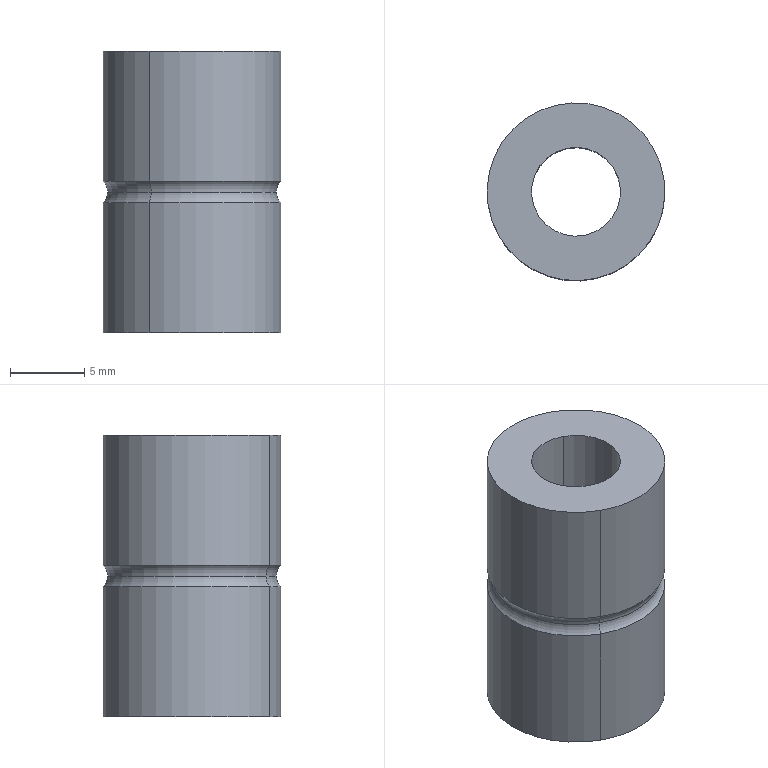Part | SolidWorks | features BaseBody 1 | 1 solid | 12 faces | box 12 x 12 x 19 mm | volume 1601 mm3 | cylinder 6 | torus 4 | plane 2 | commonest cylinder face diameters 12 x4 6 x2
STEP:
#1=CARTESIAN_POINT('',(-798.033,661.045,523.732));
#2=VERTEX_POINT('',#1);
#3=CARTESIAN_POINT('',(-792.229,671.548,523.732));
#4=VERTEX_POINT('',#3);
#5=CARTESIAN_POINT('',(-795.131,666.297,523.732));
#6=DIRECTION('',(0.,0.,1.));
#7=DIRECTION('',(-0.4837,-0.8752,0.));
#8=AXIS2_PLACEMENT_3D('',#5,#6,#7);
#9=CIRCLE('',#8,6.);
#10=EDGE_CURVE('',#2,#4,#9,.T.);
#11=ORIENTED_EDGE('',*,*,#10,.T.);
#12=CARTESIAN_POINT('',(-792.229,671.548,532.518));
#13=VERTEX_POINT('',#12);
#14=CARTESIAN_POINT('',(-792.229,671.548,532.518));
#15=DIRECTION('',(0.,0.,-1.));
#16=VECTOR('',#15,1000.);
#17=LINE('',#14,#16);
#18=EDGE_CURVE('',#13,#4,#17,.T.);
#19=ORIENTED_EDGE('',*,*,#18,.F.);
#20=CARTESIAN_POINT('',(-798.033,661.045,532.518));
#21=VERTEX_POINT('',#20);
#22=CARTESIAN_POINT('',(-795.131,666.297,532.518));
#23=DIRECTION('',(0.,0.,-1.));
#24=DIRECTION('',(0.4837,0.8752,0.));
#25=AXIS2_PLACEMENT_3D('',#22,#23,#24);
#26=CIRCLE('',#25,6.);
#27=EDGE_CURVE('',#13,#21,#26,.T.);
#28=ORIENTED_EDGE('',*,*,#27,.T.);
#29=CARTESIAN_POINT('',(-798.033,661.045,523.732));
#30=DIRECTION('',(0.,0.,1.));
#31=VECTOR('',#30,1000.);
#32=LINE('',#29,#31);
#33=EDGE_CURVE('',#2,#21,#32,.T.);
#34=ORIENTED_EDGE('',*,*,#33,.F.);
#35=EDGE_LOOP('',(#11,#19,#28,#34));
#36=FACE_OUTER_BOUND('',#35,.T.);
#37=CARTESIAN_POINT('',(-795.131,666.297,541.232));
#38=DIRECTION('',(0.,0.,-1.));
#39=DIRECTION('',(-0.4837,-0.8752,0.));
#40=AXIS2_PLACEMENT_3D('',#37,#38,#39);
#41=CYLINDRICAL_SURFACE('',#40,6.);
#42=ADVANCED_FACE('',(#36),#41,.T.);
#43=ORIENTED_EDGE('',*,*,#18,.T.);
#44=CARTESIAN_POINT('',(-795.131,666.297,523.732));
#45=DIRECTION('',(0.,0.,1.));
#46=DIRECTION('',(0.4837,0.8752,0.));
#47=AXIS2_PLACEMENT_3D('',#44,#45,#46);
#48=CIRCLE('',#47,6.);
#49=EDGE_CURVE('',#4,#2,#48,.T.);
#50=ORIENTED_EDGE('',*,*,#49,.T.);
#51=ORIENTED_EDGE('',*,*,#33,.T.);
#52=CARTESIAN_POINT('',(-795.131,666.297,532.518));
#53=DIRECTION('',(0.,0.,-1.));
#54=DIRECTION('',(-0.4837,-0.8752,0.));
#55=AXIS2_PLACEMENT_3D('',#52,#53,#54);
#56=CIRCLE('',#55,6.);
#57=EDGE_CURVE('',#21,#13,#56,.T.);
#58=ORIENTED_EDGE('',*,*,#57,.T.);
#59=EDGE_LOOP('',(#43,#50,#51,#58));
#60=FACE_OUTER_BOUND('',#59,.T.);
#61=CARTESIAN_POINT('',(-795.131,666.297,541.232));
#62=DIRECTION('',(0.,0.,-1.));
#63=DIRECTION('',(-0.4837,-0.8752,0.));
#64=AXIS2_PLACEMENT_3D('',#61,#62,#63);
#65=CYLINDRICAL_SURFACE('',#64,6.);
#66=ADVANCED_FACE('',(#60),#65,.T.);
#67=CARTESIAN_POINT('',(-792.374,671.286,533.232));
#68=VERTEX_POINT('',#67);
#69=CARTESIAN_POINT('',(-791.89,672.161,533.232));
#70=DIRECTION('',(0.8752,-0.4837,0.));
#71=DIRECTION('',(-0.4837,-0.8752,0.));
#72=AXIS2_PLACEMENT_3D('',#69,#70,#71);
#73=CIRCLE('',#72,1.);
#74=EDGE_CURVE('',#68,#13,#73,.T.);
#75=ORIENTED_EDGE('',*,*,#74,.T.);
#76=ORIENTED_EDGE('',*,*,#57,.F.);
#77=CARTESIAN_POINT('',(-797.888,661.308,533.232));
#78=VERTEX_POINT('',#77);
#79=CARTESIAN_POINT('',(-798.371,660.433,533.232));
#80=DIRECTION('',(0.8752,-0.4837,0.));
#81=DIRECTION('',(0.3386,0.6127,-0.7141));
#82=AXIS2_PLACEMENT_3D('',#79,#80,#81);
#83=CIRCLE('',#82,1.);
#84=EDGE_CURVE('',#21,#78,#83,.T.);
#85=ORIENTED_EDGE('',*,*,#84,.T.);
#86=CARTESIAN_POINT('',(-795.131,666.297,533.232));
#87=DIRECTION('',(0.,0.,1.));
#88=DIRECTION('',(0.4837,0.8752,0.));
#89=AXIS2_PLACEMENT_3D('',#86,#87,#88);
#90=CIRCLE('',#89,5.7);
#91=EDGE_CURVE('',#68,#78,#90,.T.);
#92=ORIENTED_EDGE('',*,*,#91,.F.);
#93=EDGE_LOOP('',(#75,#76,#85,#92));
#94=FACE_OUTER_BOUND('',#93,.T.);
#95=CARTESIAN_POINT('',(-795.131,666.297,533.232));
#96=DIRECTION('',(0.,0.,-1.));
#97=DIRECTION('',(-0.4837,-0.8752,0.));
#98=AXIS2_PLACEMENT_3D('',#95,#96,#97);
#99=TOROIDAL_SURFACE('',#98,6.7,1.);
#100=ADVANCED_FACE('',(#94),#99,.F.);
#101=CARTESIAN_POINT('',(-792.229,671.548,533.946));
#102=VERTEX_POINT('',#101);
#103=CARTESIAN_POINT('',(-798.033,661.045,533.946));
#104=VERTEX_POINT('',#103);
#105=CARTESIAN_POINT('',(-795.131,666.297,533.946));
#106=DIRECTION('',(0.,0.,1.));
#107=DIRECTION('',(0.4837,0.8752,0.));
#108=AXIS2_PLACEMENT_3D('',#105,#106,#107);
#109=CIRCLE('',#108,6.);
#110=EDGE_CURVE('',#102,#104,#109,.T.);
#111=ORIENTED_EDGE('',*,*,#110,.F.);
#112=CARTESIAN_POINT('',(-791.89,672.161,533.232));
#113=DIRECTION('',(-0.8752,0.4837,0.));
#114=DIRECTION('',(-0.4837,-0.8752,0.));
#115=AXIS2_PLACEMENT_3D('',#112,#113,#114);
#116=CIRCLE('',#115,1.);
#117=EDGE_CURVE('',#68,#102,#116,.T.);
#118=ORIENTED_EDGE('',*,*,#117,.F.);
#119=ORIENTED_EDGE('',*,*,#91,.T.);
#120=CARTESIAN_POINT('',(-798.371,660.433,533.232));
#121=DIRECTION('',(-0.8752,0.4837,0.));
#122=DIRECTION('',(0.3386,0.6127,0.7141));
#123=AXIS2_PLACEMENT_3D('',#120,#121,#122);
#124=CIRCLE('',#123,1.);
#125=EDGE_CURVE('',#104,#78,#124,.T.);
#126=ORIENTED_EDGE('',*,*,#125,.F.);
#127=EDGE_LOOP('',(#111,#118,#119,#126));
#128=FACE_OUTER_BOUND('',#127,.T.);
#129=CARTESIAN_POINT('',(-795.131,666.297,533.232));
#130=DIRECTION('',(0.,0.,-1.));
#131=DIRECTION('',(-0.4837,-0.8752,0.));
#132=AXIS2_PLACEMENT_3D('',#129,#130,#131);
#133=TOROIDAL_SURFACE('',#132,6.7,1.);
#134=ADVANCED_FACE('',(#128),#133,.F.);
#135=CARTESIAN_POINT('',(-795.131,666.297,533.946));
#136=DIRECTION('',(0.,0.,1.));
#137=DIRECTION('',(-0.4837,-0.8752,0.));
#138=AXIS2_PLACEMENT_3D('',#135,#136,#137);
#139=CIRCLE('',#138,6.);
#140=EDGE_CURVE('',#104,#102,#139,.T.);
#141=ORIENTED_EDGE('',*,*,#140,.F.);
#142=ORIENTED_EDGE('',*,*,#125,.T.);
#143=CARTESIAN_POINT('',(-795.131,666.297,533.232));
#144=DIRECTION('',(0.,0.,1.));
#145=DIRECTION('',(-0.4837,-0.8752,0.));
#146=AXIS2_PLACEMENT_3D('',#143,#144,#145);
#147=CIRCLE('',#146,5.7);
#148=EDGE_CURVE('',#78,#68,#147,.T.);
#149=ORIENTED_EDGE('',*,*,#148,.T.);
#150=ORIENTED_EDGE('',*,*,#117,.T.);
#151=EDGE_LOOP('',(#141,#142,#149,#150));
#152=FACE_OUTER_BOUND('',#151,.T.);
#153=CARTESIAN_POINT('',(-795.131,666.297,533.232));
#154=DIRECTION('',(0.,0.,-1.));
#155=DIRECTION('',(-0.4837,-0.8752,0.));
#156=AXIS2_PLACEMENT_3D('',#153,#154,#155);
#157=TOROIDAL_SURFACE('',#156,6.7,1.);
#158=ADVANCED_FACE('',(#152),#157,.F.);
#159=ORIENTED_EDGE('',*,*,#84,.F.);
#160=ORIENTED_EDGE('',*,*,#27,.F.);
#161=ORIENTED_EDGE('',*,*,#74,.F.);
#162=ORIENTED_EDGE('',*,*,#148,.F.);
#163=EDGE_LOOP('',(#159,#160,#161,#162));
#164=FACE_OUTER_BOUND('',#163,.T.);
#165=CARTESIAN_POINT('',(-795.131,666.297,533.232));
#166=DIRECTION('',(0.,0.,-1.));
#167=DIRECTION('',(-0.4837,-0.8752,0.));
#168=AXIS2_PLACEMENT_3D('',#165,#166,#167);
#169=TOROIDAL_SURFACE('',#168,6.7,1.);
#170=ADVANCED_FACE('',(#164),#169,.F.);
#171=ORIENTED_EDGE('',*,*,#140,.T.);
#172=CARTESIAN_POINT('',(-792.229,671.548,542.732));
#173=VERTEX_POINT('',#172);
#174=CARTESIAN_POINT('',(-792.229,671.548,542.732));
#175=DIRECTION('',(0.,0.,-1.));
#176=VECTOR('',#175,1000.);
#177=LINE('',#174,#176);
#178=EDGE_CURVE('',#173,#102,#177,.T.);
#179=ORIENTED_EDGE('',*,*,#178,.F.);
#180=CARTESIAN_POINT('',(-798.033,661.045,542.732));
#181=VERTEX_POINT('',#180);
#182=CARTESIAN_POINT('',(-795.131,666.297,542.732));
#183=DIRECTION('',(0.,0.,-1.));
#184=DIRECTION('',(0.4837,0.8752,0.));
#185=AXIS2_PLACEMENT_3D('',#182,#183,#184);
#186=CIRCLE('',#185,6.);
#187=EDGE_CURVE('',#173,#181,#186,.T.);
#188=ORIENTED_EDGE('',*,*,#187,.T.);
#189=CARTESIAN_POINT('',(-798.033,661.045,533.946));
#190=DIRECTION('',(0.,0.,1.));
#191=VECTOR('',#190,1000.);
#192=LINE('',#189,#191);
#193=EDGE_CURVE('',#104,#181,#192,.T.);
#194=ORIENTED_EDGE('',*,*,#193,.F.);
#195=EDGE_LOOP('',(#171,#179,#188,#194));
#196=FACE_OUTER_BOUND('',#195,.T.);
#197=CARTESIAN_POINT('',(-795.131,666.297,541.232));
#198=DIRECTION('',(0.,0.,-1.));
#199=DIRECTION('',(-0.4837,-0.8752,0.));
#200=AXIS2_PLACEMENT_3D('',#197,#198,#199);
#201=CYLINDRICAL_SURFACE('',#200,6.);
#202=ADVANCED_FACE('',(#196),#201,.T.);
#203=ORIENTED_EDGE('',*,*,#178,.T.);
#204=ORIENTED_EDGE('',*,*,#110,.T.);
#205=ORIENTED_EDGE('',*,*,#193,.T.);
#206=CARTESIAN_POINT('',(-795.131,666.297,542.732));
#207=DIRECTION('',(0.,0.,-1.));
#208=DIRECTION('',(-0.4837,-0.8752,0.));
#209=AXIS2_PLACEMENT_3D('',#206,#207,#208);
#210=CIRCLE('',#209,6.);
#211=EDGE_CURVE('',#181,#173,#210,.T.);
#212=ORIENTED_EDGE('',*,*,#211,.T.);
#213=EDGE_LOOP('',(#203,#204,#205,#212));
#214=FACE_OUTER_BOUND('',#213,.T.);
#215=CARTESIAN_POINT('',(-795.131,666.297,541.232));
#216=DIRECTION('',(0.,0.,-1.));
#217=DIRECTION('',(-0.4837,-0.8752,0.));
#218=AXIS2_PLACEMENT_3D('',#215,#216,#217);
#219=CYLINDRICAL_SURFACE('',#218,6.);
#220=ADVANCED_FACE('',(#214),#219,.T.);
#221=ORIENTED_EDGE('',*,*,#187,.F.);
#222=ORIENTED_EDGE('',*,*,#211,.F.);
#223=EDGE_LOOP('',(#221,#222));
#224=FACE_OUTER_BOUND('',#223,.T.);
#225=CARTESIAN_POINT('',(-796.582,663.671,542.732));
#226=VERTEX_POINT('',#225);
#227=CARTESIAN_POINT('',(-793.68,668.923,542.732));
#228=VERTEX_POINT('',#227);
#229=CARTESIAN_POINT('',(-795.131,666.297,542.732));
#230=DIRECTION('',(0.,0.,1.));
#231=DIRECTION('',(-0.4837,-0.8752,0.));
#232=AXIS2_PLACEMENT_3D('',#229,#230,#231);
#233=CIRCLE('',#232,3.);
#234=EDGE_CURVE('',#226,#228,#233,.T.);
#235=ORIENTED_EDGE('',*,*,#234,.F.);
#236=CARTESIAN_POINT('',(-795.131,666.297,542.732));
#237=DIRECTION('',(0.,0.,1.));
#238=DIRECTION('',(0.4837,0.8752,0.));
#239=AXIS2_PLACEMENT_3D('',#236,#237,#238);
#240=CIRCLE('',#239,3.);
#241=EDGE_CURVE('',#228,#226,#240,.T.);
#242=ORIENTED_EDGE('',*,*,#241,.F.);
#243=EDGE_LOOP('',(#235,#242));
#244=FACE_BOUND('',#243,.T.);
#245=CARTESIAN_POINT('',(-790.229,663.588,542.732));
#246=DIRECTION('',(0.,0.,-1.));
#247=DIRECTION('',(-0.4837,-0.8752,0.));
#248=AXIS2_PLACEMENT_3D('',#245,#246,#247);
#249=PLANE('',#248);
#250=ADVANCED_FACE('',(#224,#244),#249,.F.);
#251=CARTESIAN_POINT('',(-796.582,663.671,523.732));
#252=VERTEX_POINT('',#251);
#253=CARTESIAN_POINT('',(-793.68,668.923,523.732));
#254=VERTEX_POINT('',#253);
#255=CARTESIAN_POINT('',(-795.131,666.297,523.732));
#256=DIRECTION('',(0.,0.,-1.));
#257=DIRECTION('',(-0.4837,-0.8752,0.));
#258=AXIS2_PLACEMENT_3D('',#255,#256,#257);
#259=CIRCLE('',#258,3.);
#260=EDGE_CURVE('',#252,#254,#259,.T.);
#261=ORIENTED_EDGE('',*,*,#260,.T.);
#262=CARTESIAN_POINT('',(-793.68,668.923,523.732));
#263=DIRECTION('',(0.,0.,1.));
#264=VECTOR('',#263,1000.);
#265=LINE('',#262,#264);
#266=EDGE_CURVE('',#254,#228,#265,.T.);
#267=ORIENTED_EDGE('',*,*,#266,.T.);
#268=ORIENTED_EDGE('',*,*,#241,.T.);
#269=CARTESIAN_POINT('',(-796.582,663.671,542.732));
#270=DIRECTION('',(0.,0.,-1.));
#271=VECTOR('',#270,1000.);
#272=LINE('',#269,#271);
#273=EDGE_CURVE('',#226,#252,#272,.T.);
#274=ORIENTED_EDGE('',*,*,#273,.T.);
#275=EDGE_LOOP('',(#261,#267,#268,#274));
#276=FACE_OUTER_BOUND('',#275,.T.);
#277=CARTESIAN_POINT('',(-795.131,666.297,541.232));
#278=DIRECTION('',(0.,0.,-1.));
#279=DIRECTION('',(-0.4837,-0.8752,0.));
#280=AXIS2_PLACEMENT_3D('',#277,#278,#279);
#281=CYLINDRICAL_SURFACE('',#280,3.);
#282=ADVANCED_FACE('',(#276),#281,.F.);
#283=ORIENTED_EDGE('',*,*,#266,.F.);
#284=CARTESIAN_POINT('',(-795.131,666.297,523.732));
#285=DIRECTION('',(0.,0.,-1.));
#286=DIRECTION('',(0.4837,0.8752,0.));
#287=AXIS2_PLACEMENT_3D('',#284,#285,#286);
#288=CIRCLE('',#287,3.);
#289=EDGE_CURVE('',#254,#252,#288,.T.);
#290=ORIENTED_EDGE('',*,*,#289,.T.);
#291=ORIENTED_EDGE('',*,*,#273,.F.);
#292=ORIENTED_EDGE('',*,*,#234,.T.);
#293=EDGE_LOOP('',(#283,#290,#291,#292));
#294=FACE_OUTER_BOUND('',#293,.T.);
#295=CARTESIAN_POINT('',(-795.131,666.297,541.232));
#296=DIRECTION('',(0.,0.,-1.));
#297=DIRECTION('',(-0.4837,-0.8752,0.));
#298=AXIS2_PLACEMENT_3D('',#295,#296,#297);
#299=CYLINDRICAL_SURFACE('',#298,3.);
#300=ADVANCED_FACE('',(#294),#299,.F.);
#301=ORIENTED_EDGE('',*,*,#10,.F.);
#302=ORIENTED_EDGE('',*,*,#49,.F.);
#303=EDGE_LOOP('',(#301,#302));
#304=FACE_OUTER_BOUND('',#303,.T.);
#305=ORIENTED_EDGE('',*,*,#289,.F.);
#306=ORIENTED_EDGE('',*,*,#260,.F.);
#307=EDGE_LOOP('',(#305,#306));
#308=FACE_BOUND('',#307,.T.);
#309=CARTESIAN_POINT('',(-795.131,666.297,523.732));
#310=DIRECTION('',(0.,0.,1.));
#311=DIRECTION('',(0.4837,0.8752,0.));
#312=AXIS2_PLACEMENT_3D('',#309,#310,#311);
#313=PLANE('',#312);
#314=ADVANCED_FACE('',(#304,#308),#313,.F.);
#315=CLOSED_SHELL('',(#42,#66,#100,#134,#158,#170,#202,#220,#250,#282,#300,#314));
#316=MANIFOLD_SOLID_BREP('',#315);
#317=CARTESIAN_POINT('',(0.,0.,0.));
#318=DIRECTION('',(0.,0.,1.));
#319=DIRECTION('',(1.,0.,0.));
#320=AXIS2_PLACEMENT_3D('',#317,#318,#319);
#321=(LENGTH_UNIT()NAMED_UNIT(*)SI_UNIT(.MILLI.,.METRE.));
#322=UNCERTAINTY_MEASURE_WITH_UNIT(LENGTH_MEASURE(0.00001),#321,'','');
#323=(NAMED_UNIT(*)PLANE_ANGLE_UNIT()SI_UNIT($,.RADIAN.));
#324=(NAMED_UNIT(*)SI_UNIT($,.STERADIAN.)SOLID_ANGLE_UNIT());
#325=(GEOMETRIC_REPRESENTATION_CONTEXT(3)GLOBAL_UNCERTAINTY_ASSIGNED_CONTEXT((#322))GLOBAL_UNIT_ASSIGNED_CONTEXT((#321,#323,#324))REPRESENTATION_CONTEXT('',''));
#326=ADVANCED_BREP_SHAPE_REPRESENTATION('',(#316,#320),#325);